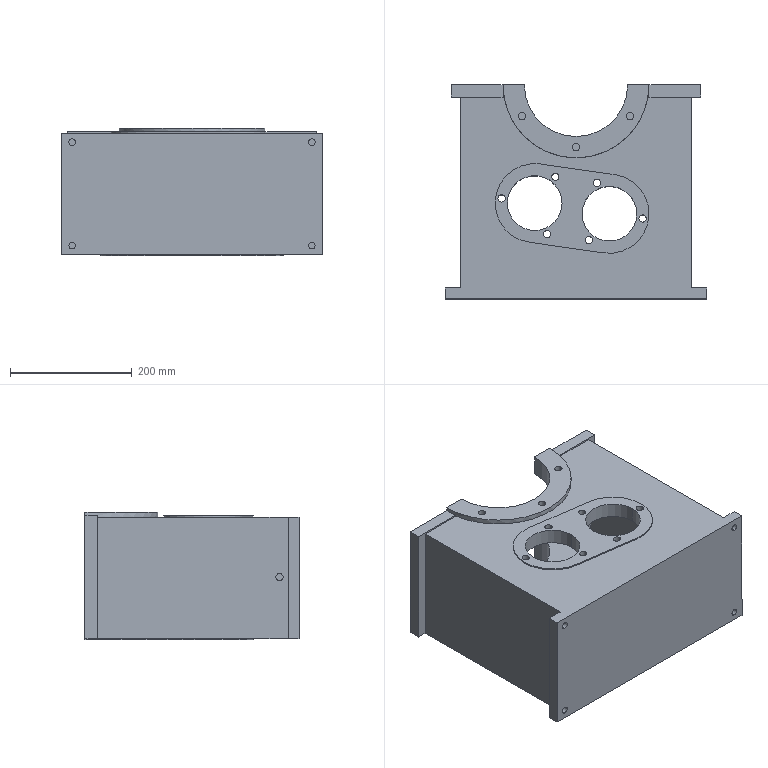Part | SolidWorks | features ICE 16, HoleWzd 12, Extrusion 1, Fillet 1 | 1 solid | 131 faces | box 430 x 352 x 210 mm | volume 7645856 mm3 | cylinder 86 | plane 45 | commonest cylinder face diameters 12 x40 130 x12 11 x8 90 x8 8 x4 16 x4